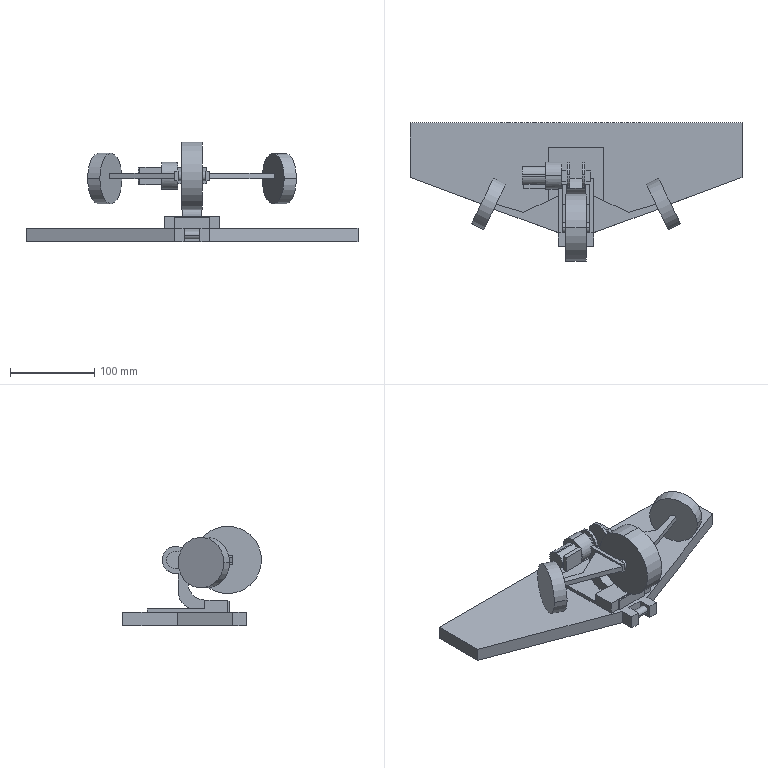Part | SolidWorks | features ICE 20, Fillet 5, Extrusion 1 | 1 solid | 123 faces | box 393.785 x 164.433 x 118.113 mm | volume 975900 mm3 | plane 92 | cylinder 31 | commonest cylinder face diameters 20 x8 30 x6 11.263 x4 60 x4 40 x3 10 x2